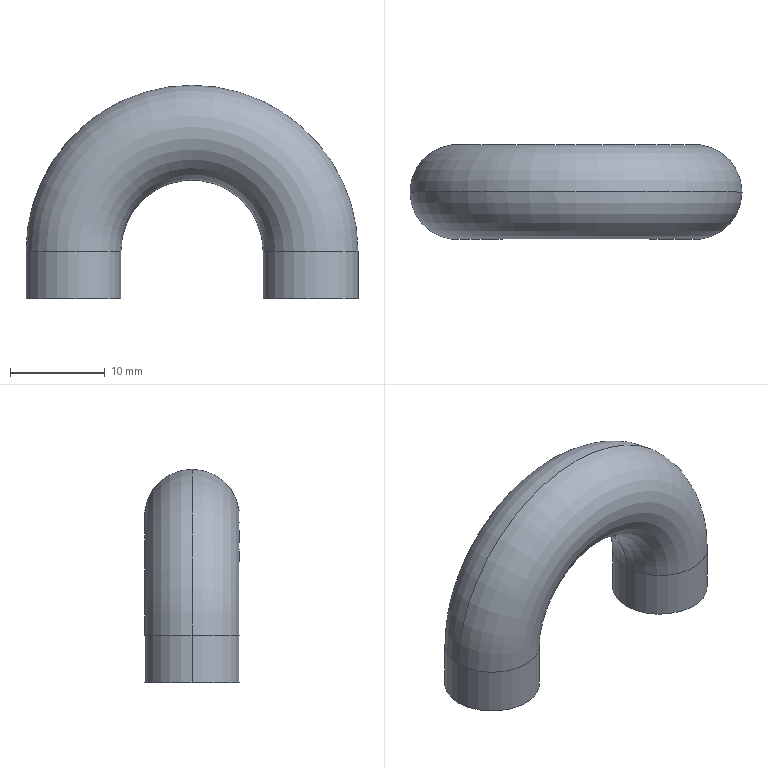Part | STEP file | connecting copper tube | 1 solid | 8 faces | box 35 x 10 x 22.5 mm | volume 3870 mm3 | cylinder 4 | torus 2 | plane 2 | commonest cylinder face diameters 10 x4
STEP:
#1=CARTESIAN_POINT('',(0.,0.,0.));
#2=DIRECTION('',(0.,0.,1.));
#3=DIRECTION('',(1.,0.,0.));
#4=AXIS2_PLACEMENT_3D('',#1,#2,#3);
#5=CARTESIAN_POINT('',(176.174,264.371,5.));
#6=VERTEX_POINT('',#5);
#7=CARTESIAN_POINT('',(186.174,264.371,5.));
#8=VERTEX_POINT('',#7);
#9=CARTESIAN_POINT('',(181.174,264.371,5.));
#10=DIRECTION('',(0.,0.,1.));
#11=DIRECTION('',(1.,0.,0.));
#12=AXIS2_PLACEMENT_3D('',#9,#10,#11);
#13=CIRCLE('',#12,5.);
#14=CARTESIAN_POINT('',(168.674,264.371,5.));
#15=DIRECTION('',(0.,-1.,0.));
#16=DIRECTION('',(0.,0.,-1.));
#17=AXIS2_PLACEMENT_3D('',#14,#15,#16);
#18=TOROIDAL_SURFACE('',#17,12.5,5.);
#19=CARTESIAN_POINT('',(1.571,6.283));
#20=DIRECTION('',(0.,-1.));
#21=VECTOR('',#20,1.);
#22=LINE('',#19,#21);
#23=(GEOMETRIC_REPRESENTATION_CONTEXT(2)PARAMETRIC_REPRESENTATION_CONTEXT()REPRESENTATION_CONTEXT('',''));
#24=DEFINITIONAL_REPRESENTATION('',(#22),#23);
#25=PCURVE('',#18,#24);
#26=CARTESIAN_POINT('',(181.174,264.371,5.));
#27=DIRECTION('',(0.,0.,-1.));
#28=DIRECTION('',(-1.,0.,0.));
#29=AXIS2_PLACEMENT_3D('',#26,#27,#28);
#30=CYLINDRICAL_SURFACE('',#29,5.);
#31=CARTESIAN_POINT('',(9.425,0.));
#32=DIRECTION('',(-1.,0.));
#33=VECTOR('',#32,1.);
#34=LINE('',#31,#33);
#35=(GEOMETRIC_REPRESENTATION_CONTEXT(2)PARAMETRIC_REPRESENTATION_CONTEXT()REPRESENTATION_CONTEXT('',''));
#36=DEFINITIONAL_REPRESENTATION('',(#34),#35);
#37=PCURVE('',#30,#36);
#38=SURFACE_CURVE('',#13,(#25,#37),.PCURVE_S1.);
#39=EDGE_CURVE('',#6,#8,#38,.T.);
#40=ORIENTED_EDGE('',*,*,#39,.T.);
#41=CARTESIAN_POINT('',(151.174,264.371,5.));
#42=VERTEX_POINT('',#41);
#43=CARTESIAN_POINT('',(168.674,264.371,5.));
#44=DIRECTION('',(0.,-1.,0.));
#45=DIRECTION('',(0.,0.,-1.));
#46=AXIS2_PLACEMENT_3D('',#43,#44,#45);
#47=CIRCLE('',#46,17.5);
#48=CARTESIAN_POINT('',(0.,0.));
#49=DIRECTION('',(1.,0.));
#50=VECTOR('',#49,1.);
#51=LINE('',#48,#50);
#52=(GEOMETRIC_REPRESENTATION_CONTEXT(2)PARAMETRIC_REPRESENTATION_CONTEXT()REPRESENTATION_CONTEXT('',''));
#53=DEFINITIONAL_REPRESENTATION('',(#51),#52);
#54=PCURVE('',#18,#53);
#55=CARTESIAN_POINT('',(168.674,264.371,5.));
#56=DIRECTION('',(0.,-1.,0.));
#57=DIRECTION('',(0.,0.,-1.));
#58=AXIS2_PLACEMENT_3D('',#55,#56,#57);
#59=TOROIDAL_SURFACE('',#58,12.5,5.);
#60=CARTESIAN_POINT('',(0.,6.283));
#61=DIRECTION('',(1.,0.));
#62=VECTOR('',#61,1.);
#63=LINE('',#60,#62);
#64=(GEOMETRIC_REPRESENTATION_CONTEXT(2)PARAMETRIC_REPRESENTATION_CONTEXT()REPRESENTATION_CONTEXT('',''));
#65=DEFINITIONAL_REPRESENTATION('',(#63),#64);
#66=PCURVE('',#59,#65);
#67=SURFACE_CURVE('',#47,(#54,#66),.PCURVE_S1.);
#68=EDGE_CURVE('',#8,#42,#67,.T.);
#69=ORIENTED_EDGE('',*,*,#68,.T.);
#70=CARTESIAN_POINT('',(161.174,264.371,5.));
#71=VERTEX_POINT('',#70);
#72=CARTESIAN_POINT('',(156.174,264.371,5.));
#73=DIRECTION('',(0.,0.,-1.));
#74=DIRECTION('',(-1.,0.,0.));
#75=AXIS2_PLACEMENT_3D('',#72,#73,#74);
#76=CIRCLE('',#75,5.);
#77=CARTESIAN_POINT('',(4.712,6.283));
#78=DIRECTION('',(0.,-1.));
#79=VECTOR('',#78,1.);
#80=LINE('',#77,#79);
#81=(GEOMETRIC_REPRESENTATION_CONTEXT(2)PARAMETRIC_REPRESENTATION_CONTEXT()REPRESENTATION_CONTEXT('',''));
#82=DEFINITIONAL_REPRESENTATION('',(#80),#81);
#83=PCURVE('',#18,#82);
#84=CARTESIAN_POINT('',(156.174,264.371,5.));
#85=DIRECTION('',(0.,0.,-1.));
#86=DIRECTION('',(-1.,0.,0.));
#87=AXIS2_PLACEMENT_3D('',#84,#85,#86);
#88=CYLINDRICAL_SURFACE('',#87,5.);
#89=CARTESIAN_POINT('',(0.,0.));
#90=DIRECTION('',(1.,0.));
#91=VECTOR('',#90,1.);
#92=LINE('',#89,#91);
#93=(GEOMETRIC_REPRESENTATION_CONTEXT(2)PARAMETRIC_REPRESENTATION_CONTEXT()REPRESENTATION_CONTEXT('',''));
#94=DEFINITIONAL_REPRESENTATION('',(#92),#93);
#95=PCURVE('',#88,#94);
#96=SURFACE_CURVE('',#76,(#83,#95),.PCURVE_S1.);
#97=EDGE_CURVE('',#71,#42,#96,.T.);
#98=ORIENTED_EDGE('',*,*,#97,.F.);
#99=CARTESIAN_POINT('',(168.674,264.371,5.));
#100=DIRECTION('',(0.,-1.,0.));
#101=DIRECTION('',(0.,0.,-1.));
#102=AXIS2_PLACEMENT_3D('',#99,#100,#101);
#103=CIRCLE('',#102,7.5);
#104=CARTESIAN_POINT('',(0.,3.142));
#105=DIRECTION('',(1.,0.));
#106=VECTOR('',#105,1.);
#107=LINE('',#104,#106);
#108=(GEOMETRIC_REPRESENTATION_CONTEXT(2)PARAMETRIC_REPRESENTATION_CONTEXT()REPRESENTATION_CONTEXT('',''));
#109=DEFINITIONAL_REPRESENTATION('',(#107),#108);
#110=PCURVE('',#18,#109);
#111=CARTESIAN_POINT('',(0.,3.142));
#112=DIRECTION('',(1.,0.));
#113=VECTOR('',#112,1.);
#114=LINE('',#111,#113);
#115=(GEOMETRIC_REPRESENTATION_CONTEXT(2)PARAMETRIC_REPRESENTATION_CONTEXT()REPRESENTATION_CONTEXT('',''));
#116=DEFINITIONAL_REPRESENTATION('',(#114),#115);
#117=PCURVE('',#59,#116);
#118=SURFACE_CURVE('',#103,(#110,#117),.PCURVE_S1.);
#119=EDGE_CURVE('',#6,#71,#118,.T.);
#120=ORIENTED_EDGE('',*,*,#119,.F.);
#121=EDGE_LOOP('',(#40,#69,#98,#120));
#122=FACE_BOUND('',#121,.T.);
#123=ADVANCED_FACE('',(#122),#18,.T.);
#124=CARTESIAN_POINT('',(181.174,264.371,5.));
#125=DIRECTION('',(0.,0.,1.));
#126=DIRECTION('',(1.,0.,0.));
#127=AXIS2_PLACEMENT_3D('',#124,#125,#126);
#128=CIRCLE('',#127,5.);
#129=CARTESIAN_POINT('',(181.174,264.371,5.));
#130=DIRECTION('',(0.,0.,-1.));
#131=DIRECTION('',(-1.,0.,0.));
#132=AXIS2_PLACEMENT_3D('',#129,#130,#131);
#133=CYLINDRICAL_SURFACE('',#132,5.);
#134=CARTESIAN_POINT('',(3.142,0.));
#135=DIRECTION('',(-1.,0.));
#136=VECTOR('',#135,1.);
#137=LINE('',#134,#136);
#138=(GEOMETRIC_REPRESENTATION_CONTEXT(2)PARAMETRIC_REPRESENTATION_CONTEXT()REPRESENTATION_CONTEXT('',''));
#139=DEFINITIONAL_REPRESENTATION('',(#137),#138);
#140=PCURVE('',#133,#139);
#141=CARTESIAN_POINT('',(1.571,6.283));
#142=DIRECTION('',(0.,-1.));
#143=VECTOR('',#142,1.);
#144=LINE('',#141,#143);
#145=(GEOMETRIC_REPRESENTATION_CONTEXT(2)PARAMETRIC_REPRESENTATION_CONTEXT()REPRESENTATION_CONTEXT('',''));
#146=DEFINITIONAL_REPRESENTATION('',(#144),#145);
#147=PCURVE('',#59,#146);
#148=SURFACE_CURVE('',#128,(#140,#147),.PCURVE_S1.);
#149=EDGE_CURVE('',#8,#6,#148,.T.);
#150=ORIENTED_EDGE('',*,*,#149,.F.);
#151=CARTESIAN_POINT('',(186.174,264.371,0.));
#152=VERTEX_POINT('',#151);
#153=CARTESIAN_POINT('',(186.174,264.371,5.));
#154=DIRECTION('',(0.,0.,-1.));
#155=VECTOR('',#154,1.);
#156=LINE('',#153,#155);
#157=CARTESIAN_POINT('',(3.142,0.));
#158=DIRECTION('',(0.,1.));
#159=VECTOR('',#158,1.);
#160=LINE('',#157,#159);
#161=(GEOMETRIC_REPRESENTATION_CONTEXT(2)PARAMETRIC_REPRESENTATION_CONTEXT()REPRESENTATION_CONTEXT('',''));
#162=DEFINITIONAL_REPRESENTATION('',(#160),#161);
#163=PCURVE('',#133,#162);
#164=CARTESIAN_POINT('',(3.142,0.));
#165=DIRECTION('',(0.,1.));
#166=VECTOR('',#165,1.);
#167=LINE('',#164,#166);
#168=(GEOMETRIC_REPRESENTATION_CONTEXT(2)PARAMETRIC_REPRESENTATION_CONTEXT()REPRESENTATION_CONTEXT('',''));
#169=DEFINITIONAL_REPRESENTATION('',(#167),#168);
#170=PCURVE('',#30,#169);
#171=SURFACE_CURVE('',#156,(#163,#170),.PCURVE_S1.);
#172=EDGE_CURVE('',#8,#152,#171,.T.);
#173=ORIENTED_EDGE('',*,*,#172,.T.);
#174=CARTESIAN_POINT('',(176.174,264.371,0.));
#175=VERTEX_POINT('',#174);
#176=CARTESIAN_POINT('',(181.174,264.371,0.));
#177=DIRECTION('',(0.,0.,1.));
#178=DIRECTION('',(1.,0.,0.));
#179=AXIS2_PLACEMENT_3D('',#176,#177,#178);
#180=CIRCLE('',#179,5.);
#181=CARTESIAN_POINT('',(3.142,5.));
#182=DIRECTION('',(-1.,0.));
#183=VECTOR('',#182,1.);
#184=LINE('',#181,#183);
#185=(GEOMETRIC_REPRESENTATION_CONTEXT(2)PARAMETRIC_REPRESENTATION_CONTEXT()REPRESENTATION_CONTEXT('',''));
#186=DEFINITIONAL_REPRESENTATION('',(#184),#185);
#187=PCURVE('',#133,#186);
#188=CARTESIAN_POINT('',(181.174,264.371,0.));
#189=DIRECTION('',(0.,0.,1.));
#190=DIRECTION('',(1.,0.,0.));
#191=AXIS2_PLACEMENT_3D('',#188,#189,#190);
#192=PLANE('',#191);
#193=CARTESIAN_POINT('',(0.,0.));
#194=DIRECTION('',(1.,0.));
#195=AXIS2_PLACEMENT_2D('',#193,#194);
#196=CIRCLE('',#195,5.);
#197=(GEOMETRIC_REPRESENTATION_CONTEXT(2)PARAMETRIC_REPRESENTATION_CONTEXT()REPRESENTATION_CONTEXT('',''));
#198=DEFINITIONAL_REPRESENTATION('',(#196),#197);
#199=PCURVE('',#192,#198);
#200=SURFACE_CURVE('',#180,(#187,#199),.PCURVE_S1.);
#201=EDGE_CURVE('',#152,#175,#200,.T.);
#202=ORIENTED_EDGE('',*,*,#201,.T.);
#203=CARTESIAN_POINT('',(176.174,264.371,5.));
#204=DIRECTION('',(0.,0.,-1.));
#205=VECTOR('',#204,1.);
#206=LINE('',#203,#205);
#207=CARTESIAN_POINT('',(0.,0.));
#208=DIRECTION('',(0.,1.));
#209=VECTOR('',#208,1.);
#210=LINE('',#207,#209);
#211=(GEOMETRIC_REPRESENTATION_CONTEXT(2)PARAMETRIC_REPRESENTATION_CONTEXT()REPRESENTATION_CONTEXT('',''));
#212=DEFINITIONAL_REPRESENTATION('',(#210),#211);
#213=PCURVE('',#133,#212);
#214=CARTESIAN_POINT('',(6.283,0.));
#215=DIRECTION('',(0.,1.));
#216=VECTOR('',#215,1.);
#217=LINE('',#214,#216);
#218=(GEOMETRIC_REPRESENTATION_CONTEXT(2)PARAMETRIC_REPRESENTATION_CONTEXT()REPRESENTATION_CONTEXT('',''));
#219=DEFINITIONAL_REPRESENTATION('',(#217),#218);
#220=PCURVE('',#30,#219);
#221=SURFACE_CURVE('',#206,(#213,#220),.PCURVE_S1.);
#222=EDGE_CURVE('',#6,#175,#221,.T.);
#223=ORIENTED_EDGE('',*,*,#222,.F.);
#224=EDGE_LOOP('',(#150,#173,#202,#223));
#225=FACE_BOUND('',#224,.T.);
#226=ADVANCED_FACE('',(#225),#133,.T.);
#227=CARTESIAN_POINT('',(156.174,264.371,5.));
#228=DIRECTION('',(0.,0.,-1.));
#229=DIRECTION('',(-1.,0.,0.));
#230=AXIS2_PLACEMENT_3D('',#227,#228,#229);
#231=CIRCLE('',#230,5.);
#232=CARTESIAN_POINT('',(156.174,264.371,5.));
#233=DIRECTION('',(0.,0.,-1.));
#234=DIRECTION('',(-1.,0.,0.));
#235=AXIS2_PLACEMENT_3D('',#232,#233,#234);
#236=CYLINDRICAL_SURFACE('',#235,5.);
#237=CARTESIAN_POINT('',(0.,0.));
#238=DIRECTION('',(1.,0.));
#239=VECTOR('',#238,1.);
#240=LINE('',#237,#239);
#241=(GEOMETRIC_REPRESENTATION_CONTEXT(2)PARAMETRIC_REPRESENTATION_CONTEXT()REPRESENTATION_CONTEXT('',''));
#242=DEFINITIONAL_REPRESENTATION('',(#240),#241);
#243=PCURVE('',#236,#242);
#244=CARTESIAN_POINT('',(4.712,6.283));
#245=DIRECTION('',(0.,-1.));
#246=VECTOR('',#245,1.);
#247=LINE('',#244,#246);
#248=(GEOMETRIC_REPRESENTATION_CONTEXT(2)PARAMETRIC_REPRESENTATION_CONTEXT()REPRESENTATION_CONTEXT('',''));
#249=DEFINITIONAL_REPRESENTATION('',(#247),#248);
#250=PCURVE('',#59,#249);
#251=SURFACE_CURVE('',#231,(#243,#250),.PCURVE_S1.);
#252=EDGE_CURVE('',#42,#71,#251,.T.);
#253=ORIENTED_EDGE('',*,*,#252,.T.);
#254=CARTESIAN_POINT('',(161.174,264.371,0.));
#255=VERTEX_POINT('',#254);
#256=CARTESIAN_POINT('',(161.174,264.371,5.));
#257=DIRECTION('',(0.,0.,-1.));
#258=VECTOR('',#257,1.);
#259=LINE('',#256,#258);
#260=CARTESIAN_POINT('',(3.142,0.));
#261=DIRECTION('',(0.,1.));
#262=VECTOR('',#261,1.);
#263=LINE('',#260,#262);
#264=(GEOMETRIC_REPRESENTATION_CONTEXT(2)PARAMETRIC_REPRESENTATION_CONTEXT()REPRESENTATION_CONTEXT('',''));
#265=DEFINITIONAL_REPRESENTATION('',(#263),#264);
#266=PCURVE('',#236,#265);
#267=CARTESIAN_POINT('',(3.142,0.));
#268=DIRECTION('',(0.,1.));
#269=VECTOR('',#268,1.);
#270=LINE('',#267,#269);
#271=(GEOMETRIC_REPRESENTATION_CONTEXT(2)PARAMETRIC_REPRESENTATION_CONTEXT()REPRESENTATION_CONTEXT('',''));
#272=DEFINITIONAL_REPRESENTATION('',(#270),#271);
#273=PCURVE('',#88,#272);
#274=SURFACE_CURVE('',#259,(#266,#273),.PCURVE_S1.);
#275=EDGE_CURVE('',#71,#255,#274,.T.);
#276=ORIENTED_EDGE('',*,*,#275,.T.);
#277=CARTESIAN_POINT('',(151.174,264.371,0.));
#278=VERTEX_POINT('',#277);
#279=CARTESIAN_POINT('',(156.174,264.371,0.));
#280=DIRECTION('',(0.,0.,-1.));
#281=DIRECTION('',(-1.,0.,0.));
#282=AXIS2_PLACEMENT_3D('',#279,#280,#281);
#283=CIRCLE('',#282,5.);
#284=CARTESIAN_POINT('',(0.,5.));
#285=DIRECTION('',(1.,0.));
#286=VECTOR('',#285,1.);
#287=LINE('',#284,#286);
#288=(GEOMETRIC_REPRESENTATION_CONTEXT(2)PARAMETRIC_REPRESENTATION_CONTEXT()REPRESENTATION_CONTEXT('',''));
#289=DEFINITIONAL_REPRESENTATION('',(#287),#288);
#290=PCURVE('',#236,#289);
#291=CARTESIAN_POINT('',(156.174,264.371,0.));
#292=DIRECTION('',(0.,0.,-1.));
#293=DIRECTION('',(-1.,0.,0.));
#294=AXIS2_PLACEMENT_3D('',#291,#292,#293);
#295=PLANE('',#294);
#296=CARTESIAN_POINT('',(0.,0.));
#297=DIRECTION('',(1.,0.));
#298=AXIS2_PLACEMENT_2D('',#296,#297);
#299=CIRCLE('',#298,5.);
#300=(GEOMETRIC_REPRESENTATION_CONTEXT(2)PARAMETRIC_REPRESENTATION_CONTEXT()REPRESENTATION_CONTEXT('',''));
#301=DEFINITIONAL_REPRESENTATION('',(#299),#300);
#302=PCURVE('',#295,#301);
#303=SURFACE_CURVE('',#283,(#290,#302),.PCURVE_S1.);
#304=EDGE_CURVE('',#278,#255,#303,.T.);
#305=ORIENTED_EDGE('',*,*,#304,.F.);
#306=CARTESIAN_POINT('',(151.174,264.371,5.));
#307=DIRECTION('',(0.,0.,-1.));
#308=VECTOR('',#307,1.);
#309=LINE('',#306,#308);
#310=CARTESIAN_POINT('',(0.,0.));
#311=DIRECTION('',(0.,1.));
#312=VECTOR('',#311,1.);
#313=LINE('',#310,#312);
#314=(GEOMETRIC_REPRESENTATION_CONTEXT(2)PARAMETRIC_REPRESENTATION_CONTEXT()REPRESENTATION_CONTEXT('',''));
#315=DEFINITIONAL_REPRESENTATION('',(#313),#314);
#316=PCURVE('',#236,#315);
#317=CARTESIAN_POINT('',(6.283,0.));
#318=DIRECTION('',(0.,1.));
#319=VECTOR('',#318,1.);
#320=LINE('',#317,#319);
#321=(GEOMETRIC_REPRESENTATION_CONTEXT(2)PARAMETRIC_REPRESENTATION_CONTEXT()REPRESENTATION_CONTEXT('',''));
#322=DEFINITIONAL_REPRESENTATION('',(#320),#321);
#323=PCURVE('',#88,#322);
#324=SURFACE_CURVE('',#309,(#316,#323),.PCURVE_S1.);
#325=EDGE_CURVE('',#42,#278,#324,.T.);
#326=ORIENTED_EDGE('',*,*,#325,.F.);
#327=EDGE_LOOP('',(#253,#276,#305,#326));
#328=FACE_BOUND('',#327,.T.);
#329=ADVANCED_FACE('',(#328),#236,.T.);
#330=ORIENTED_EDGE('',*,*,#275,.F.);
#331=ORIENTED_EDGE('',*,*,#97,.T.);
#332=ORIENTED_EDGE('',*,*,#325,.T.);
#333=CARTESIAN_POINT('',(156.174,264.371,0.));
#334=DIRECTION('',(0.,0.,-1.));
#335=DIRECTION('',(-1.,0.,0.));
#336=AXIS2_PLACEMENT_3D('',#333,#334,#335);
#337=CIRCLE('',#336,5.);
#338=CARTESIAN_POINT('',(0.,5.));
#339=DIRECTION('',(1.,0.));
#340=VECTOR('',#339,1.);
#341=LINE('',#338,#340);
#342=(GEOMETRIC_REPRESENTATION_CONTEXT(2)PARAMETRIC_REPRESENTATION_CONTEXT()REPRESENTATION_CONTEXT('',''));
#343=DEFINITIONAL_REPRESENTATION('',(#341),#342);
#344=PCURVE('',#88,#343);
#345=CARTESIAN_POINT('',(0.,0.));
#346=DIRECTION('',(1.,0.));
#347=AXIS2_PLACEMENT_2D('',#345,#346);
#348=CIRCLE('',#347,5.);
#349=(GEOMETRIC_REPRESENTATION_CONTEXT(2)PARAMETRIC_REPRESENTATION_CONTEXT()REPRESENTATION_CONTEXT('',''));
#350=DEFINITIONAL_REPRESENTATION('',(#348),#349);
#351=PCURVE('',#295,#350);
#352=SURFACE_CURVE('',#337,(#344,#351),.PCURVE_S1.);
#353=EDGE_CURVE('',#255,#278,#352,.T.);
#354=ORIENTED_EDGE('',*,*,#353,.F.);
#355=EDGE_LOOP('',(#330,#331,#332,#354));
#356=FACE_BOUND('',#355,.T.);
#357=ADVANCED_FACE('',(#356),#88,.T.);
#358=ORIENTED_EDGE('',*,*,#68,.F.);
#359=ORIENTED_EDGE('',*,*,#149,.T.);
#360=ORIENTED_EDGE('',*,*,#119,.T.);
#361=ORIENTED_EDGE('',*,*,#252,.F.);
#362=EDGE_LOOP('',(#358,#359,#360,#361));
#363=FACE_BOUND('',#362,.T.);
#364=ADVANCED_FACE('',(#363),#59,.T.);
#365=ORIENTED_EDGE('',*,*,#172,.F.);
#366=ORIENTED_EDGE('',*,*,#39,.F.);
#367=ORIENTED_EDGE('',*,*,#222,.T.);
#368=CARTESIAN_POINT('',(181.174,264.371,0.));
#369=DIRECTION('',(0.,0.,1.));
#370=DIRECTION('',(1.,0.,0.));
#371=AXIS2_PLACEMENT_3D('',#368,#369,#370);
#372=CIRCLE('',#371,5.);
#373=CARTESIAN_POINT('',(9.425,5.));
#374=DIRECTION('',(-1.,0.));
#375=VECTOR('',#374,1.);
#376=LINE('',#373,#375);
#377=(GEOMETRIC_REPRESENTATION_CONTEXT(2)PARAMETRIC_REPRESENTATION_CONTEXT()REPRESENTATION_CONTEXT('',''));
#378=DEFINITIONAL_REPRESENTATION('',(#376),#377);
#379=PCURVE('',#30,#378);
#380=CARTESIAN_POINT('',(0.,0.));
#381=DIRECTION('',(1.,0.));
#382=AXIS2_PLACEMENT_2D('',#380,#381);
#383=CIRCLE('',#382,5.);
#384=(GEOMETRIC_REPRESENTATION_CONTEXT(2)PARAMETRIC_REPRESENTATION_CONTEXT()REPRESENTATION_CONTEXT('',''));
#385=DEFINITIONAL_REPRESENTATION('',(#383),#384);
#386=PCURVE('',#192,#385);
#387=SURFACE_CURVE('',#372,(#379,#386),.PCURVE_S1.);
#388=EDGE_CURVE('',#175,#152,#387,.T.);
#389=ORIENTED_EDGE('',*,*,#388,.T.);
#390=EDGE_LOOP('',(#365,#366,#367,#389));
#391=FACE_BOUND('',#390,.T.);
#392=ADVANCED_FACE('',(#391),#30,.T.);
#393=ORIENTED_EDGE('',*,*,#304,.T.);
#394=ORIENTED_EDGE('',*,*,#353,.T.);
#395=EDGE_LOOP('',(#393,#394));
#396=FACE_BOUND('',#395,.T.);
#397=ADVANCED_FACE('',(#396),#295,.T.);
#398=ORIENTED_EDGE('',*,*,#388,.F.);
#399=ORIENTED_EDGE('',*,*,#201,.F.);
#400=EDGE_LOOP('',(#398,#399));
#401=FACE_BOUND('',#400,.T.);
#402=ADVANCED_FACE('',(#401),#192,.F.);
#403=CLOSED_SHELL('',(#123,#226,#329,#357,#364,#392,#397,#402));
#404=MANIFOLD_SOLID_BREP('',#403);
#405=(LENGTH_UNIT()NAMED_UNIT(*)SI_UNIT(.MILLI.,.METRE.));
#406=UNCERTAINTY_MEASURE_WITH_UNIT(LENGTH_MEASURE(0.0000001),#405,'','');
#407=(NAMED_UNIT(*)PLANE_ANGLE_UNIT()SI_UNIT($,.RADIAN.));
#408=(NAMED_UNIT(*)SI_UNIT($,.STERADIAN.)SOLID_ANGLE_UNIT());
#409=(GEOMETRIC_REPRESENTATION_CONTEXT(3)GLOBAL_UNCERTAINTY_ASSIGNED_CONTEXT((#406))GLOBAL_UNIT_ASSIGNED_CONTEXT((#405,#407,#408))REPRESENTATION_CONTEXT('',''));
#410=ADVANCED_BREP_SHAPE_REPRESENTATION('',(#4,#404),#409);